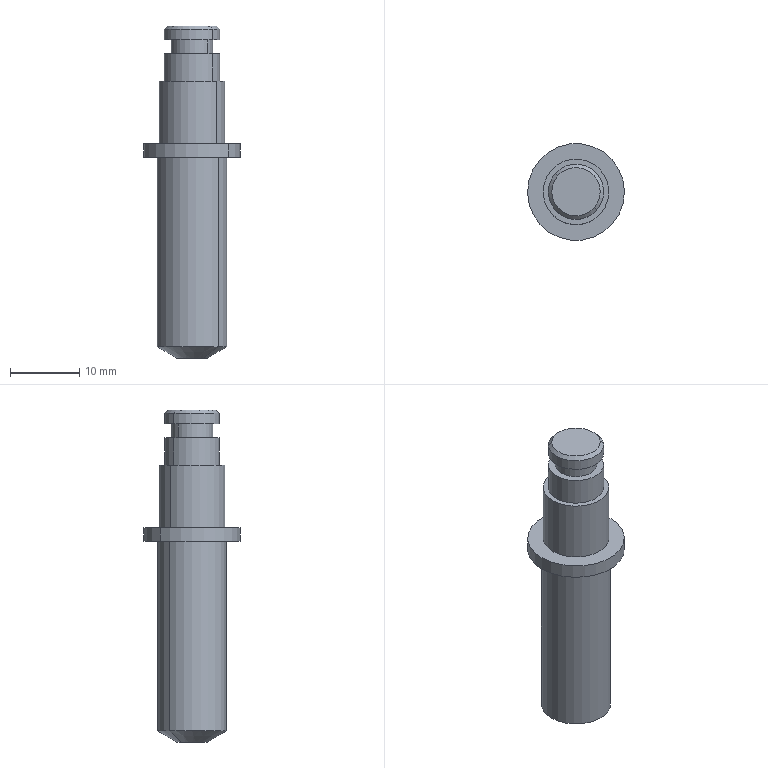Part | SolidWorks | features BaseBody 1 | 1 solid | 23 faces | box 14 x 14 x 48 mm | volume 3521 mm3 | cylinder 12 | plane 7 | cone 4 | commonest cylinder face diameters 8 x4 6 x2 9.5 x2 10 x2 14 x2
STEP:
#1=CARTESIAN_POINT('',(169.864,2.303,72.65));
#2=VERTEX_POINT('',#1);
#3=CARTESIAN_POINT('',(175.136,-2.303,72.65));
#4=VERTEX_POINT('',#3);
#5=CARTESIAN_POINT('',(172.5,0.,72.65));
#6=DIRECTION('',(0.,0.,1.));
#7=DIRECTION('',(0.7531,-0.6579,0.));
#8=AXIS2_PLACEMENT_3D('',#5,#6,#7);
#9=CIRCLE('',#8,3.5);
#10=EDGE_CURVE('',#2,#4,#9,.T.);
#11=ORIENTED_EDGE('',*,*,#10,.F.);
#12=CARTESIAN_POINT('',(169.488,2.632,72.15));
#13=VERTEX_POINT('',#12);
#14=CARTESIAN_POINT('',(169.488,2.632,72.15));
#15=DIRECTION('',(-0.5325,0.4652,-0.7071));
#16=VECTOR('',#15,1000.);
#17=LINE('',#14,#16);
#18=EDGE_CURVE('',#2,#13,#17,.T.);
#19=ORIENTED_EDGE('',*,*,#18,.T.);
#20=CARTESIAN_POINT('',(175.512,-2.632,72.15));
#21=VERTEX_POINT('',#20);
#22=CARTESIAN_POINT('',(172.5,0.,72.15));
#23=DIRECTION('',(0.,0.,-1.));
#24=DIRECTION('',(0.7531,-0.6579,0.));
#25=AXIS2_PLACEMENT_3D('',#22,#23,#24);
#26=CIRCLE('',#25,4.);
#27=EDGE_CURVE('',#21,#13,#26,.T.);
#28=ORIENTED_EDGE('',*,*,#27,.F.);
#29=CARTESIAN_POINT('',(175.512,-2.632,72.15));
#30=DIRECTION('',(0.5325,-0.4652,-0.7071));
#31=VECTOR('',#30,1000.);
#32=LINE('',#29,#31);
#33=EDGE_CURVE('',#4,#21,#32,.T.);
#34=ORIENTED_EDGE('',*,*,#33,.F.);
#35=EDGE_LOOP('',(#11,#19,#28,#34));
#36=FACE_OUTER_BOUND('',#35,.T.);
#37=CARTESIAN_POINT('',(172.5,0.,72.15));
#38=DIRECTION('',(0.,0.,-1.));
#39=DIRECTION('',(0.7531,-0.6579,0.));
#40=AXIS2_PLACEMENT_3D('',#37,#38,#39);
#41=CONICAL_SURFACE('',#40,4.,0.7854);
#42=ADVANCED_FACE('',(#36),#41,.T.);
#43=ORIENTED_EDGE('',*,*,#27,.T.);
#44=CARTESIAN_POINT('',(169.488,2.632,70.65));
#45=VERTEX_POINT('',#44);
#46=CARTESIAN_POINT('',(169.488,2.632,21.94));
#47=DIRECTION('',(0.,0.,-1.));
#48=VECTOR('',#47,1000.);
#49=LINE('',#46,#48);
#50=EDGE_CURVE('',#13,#45,#49,.T.);
#51=ORIENTED_EDGE('',*,*,#50,.T.);
#52=CARTESIAN_POINT('',(175.512,-2.632,70.65));
#53=VERTEX_POINT('',#52);
#54=CARTESIAN_POINT('',(172.5,0.,70.65));
#55=DIRECTION('',(0.,0.,-1.));
#56=DIRECTION('',(0.7531,-0.6579,0.));
#57=AXIS2_PLACEMENT_3D('',#54,#55,#56);
#58=CIRCLE('',#57,4.);
#59=EDGE_CURVE('',#53,#45,#58,.T.);
#60=ORIENTED_EDGE('',*,*,#59,.F.);
#61=CARTESIAN_POINT('',(175.512,-2.632,21.94));
#62=DIRECTION('',(0.,0.,-1.));
#63=VECTOR('',#62,1000.);
#64=LINE('',#61,#63);
#65=EDGE_CURVE('',#21,#53,#64,.T.);
#66=ORIENTED_EDGE('',*,*,#65,.F.);
#67=EDGE_LOOP('',(#43,#51,#60,#66));
#68=FACE_OUTER_BOUND('',#67,.T.);
#69=CARTESIAN_POINT('',(172.5,0.,21.94));
#70=DIRECTION('',(0.,0.,-1.));
#71=DIRECTION('',(0.7531,-0.6579,0.));
#72=AXIS2_PLACEMENT_3D('',#69,#70,#71);
#73=CYLINDRICAL_SURFACE('',#72,4.);
#74=ADVANCED_FACE('',(#68),#73,.T.);
#75=CARTESIAN_POINT('',(174.759,-1.974,70.65));
#76=VERTEX_POINT('',#75);
#77=CARTESIAN_POINT('',(170.241,1.974,70.65));
#78=VERTEX_POINT('',#77);
#79=CARTESIAN_POINT('',(172.5,0.,70.65));
#80=DIRECTION('',(0.,0.,-1.));
#81=DIRECTION('',(0.7531,-0.6579,0.));
#82=AXIS2_PLACEMENT_3D('',#79,#80,#81);
#83=CIRCLE('',#82,3.);
#84=EDGE_CURVE('',#76,#78,#83,.T.);
#85=ORIENTED_EDGE('',*,*,#84,.T.);
#86=CARTESIAN_POINT('',(170.241,1.974,68.65));
#87=VERTEX_POINT('',#86);
#88=CARTESIAN_POINT('',(170.241,1.974,21.94));
#89=DIRECTION('',(0.,0.,-1.));
#90=VECTOR('',#89,1000.);
#91=LINE('',#88,#90);
#92=EDGE_CURVE('',#78,#87,#91,.T.);
#93=ORIENTED_EDGE('',*,*,#92,.T.);
#94=CARTESIAN_POINT('',(174.759,-1.974,68.65));
#95=VERTEX_POINT('',#94);
#96=CARTESIAN_POINT('',(172.5,0.,68.65));
#97=DIRECTION('',(0.,0.,-1.));
#98=DIRECTION('',(0.7531,-0.6579,0.));
#99=AXIS2_PLACEMENT_3D('',#96,#97,#98);
#100=CIRCLE('',#99,3.);
#101=EDGE_CURVE('',#95,#87,#100,.T.);
#102=ORIENTED_EDGE('',*,*,#101,.F.);
#103=CARTESIAN_POINT('',(174.759,-1.974,21.94));
#104=DIRECTION('',(0.,0.,-1.));
#105=VECTOR('',#104,1000.);
#106=LINE('',#103,#105);
#107=EDGE_CURVE('',#76,#95,#106,.T.);
#108=ORIENTED_EDGE('',*,*,#107,.F.);
#109=EDGE_LOOP('',(#85,#93,#102,#108));
#110=FACE_OUTER_BOUND('',#109,.T.);
#111=CARTESIAN_POINT('',(172.5,0.,21.94));
#112=DIRECTION('',(0.,0.,-1.));
#113=DIRECTION('',(0.7531,-0.6579,0.));
#114=AXIS2_PLACEMENT_3D('',#111,#112,#113);
#115=CYLINDRICAL_SURFACE('',#114,3.);
#116=ADVANCED_FACE('',(#110),#115,.T.);
#117=CARTESIAN_POINT('',(175.512,-2.632,68.65));
#118=VERTEX_POINT('',#117);
#119=CARTESIAN_POINT('',(169.488,2.632,68.65));
#120=VERTEX_POINT('',#119);
#121=CARTESIAN_POINT('',(172.5,0.,68.65));
#122=DIRECTION('',(0.,0.,-1.));
#123=DIRECTION('',(0.7531,-0.6579,0.));
#124=AXIS2_PLACEMENT_3D('',#121,#122,#123);
#125=CIRCLE('',#124,4.);
#126=EDGE_CURVE('',#118,#120,#125,.T.);
#127=ORIENTED_EDGE('',*,*,#126,.T.);
#128=CARTESIAN_POINT('',(169.488,2.632,64.65));
#129=VERTEX_POINT('',#128);
#130=CARTESIAN_POINT('',(169.488,2.632,21.94));
#131=DIRECTION('',(0.,0.,-1.));
#132=VECTOR('',#131,1000.);
#133=LINE('',#130,#132);
#134=EDGE_CURVE('',#120,#129,#133,.T.);
#135=ORIENTED_EDGE('',*,*,#134,.T.);
#136=CARTESIAN_POINT('',(175.512,-2.632,64.65));
#137=VERTEX_POINT('',#136);
#138=CARTESIAN_POINT('',(172.5,0.,64.65));
#139=DIRECTION('',(0.,0.,-1.));
#140=DIRECTION('',(0.7531,-0.6579,0.));
#141=AXIS2_PLACEMENT_3D('',#138,#139,#140);
#142=CIRCLE('',#141,4.);
#143=EDGE_CURVE('',#137,#129,#142,.T.);
#144=ORIENTED_EDGE('',*,*,#143,.F.);
#145=CARTESIAN_POINT('',(175.512,-2.632,21.94));
#146=DIRECTION('',(0.,0.,-1.));
#147=VECTOR('',#146,1000.);
#148=LINE('',#145,#147);
#149=EDGE_CURVE('',#118,#137,#148,.T.);
#150=ORIENTED_EDGE('',*,*,#149,.F.);
#151=EDGE_LOOP('',(#127,#135,#144,#150));
#152=FACE_OUTER_BOUND('',#151,.T.);
#153=CARTESIAN_POINT('',(172.5,0.,21.94));
#154=DIRECTION('',(0.,0.,-1.));
#155=DIRECTION('',(0.7531,-0.6579,0.));
#156=AXIS2_PLACEMENT_3D('',#153,#154,#155);
#157=CYLINDRICAL_SURFACE('',#156,4.);
#158=ADVANCED_FACE('',(#152),#157,.T.);
#159=CARTESIAN_POINT('',(176.077,-3.125,64.65));
#160=VERTEX_POINT('',#159);
#161=CARTESIAN_POINT('',(168.923,3.125,64.65));
#162=VERTEX_POINT('',#161);
#163=CARTESIAN_POINT('',(172.5,0.,64.65));
#164=DIRECTION('',(0.,0.,-1.));
#165=DIRECTION('',(0.7531,-0.6579,0.));
#166=AXIS2_PLACEMENT_3D('',#163,#164,#165);
#167=CIRCLE('',#166,4.75);
#168=EDGE_CURVE('',#160,#162,#167,.T.);
#169=ORIENTED_EDGE('',*,*,#168,.T.);
#170=CARTESIAN_POINT('',(168.923,3.125,55.65));
#171=VERTEX_POINT('',#170);
#172=CARTESIAN_POINT('',(168.923,3.125,21.94));
#173=DIRECTION('',(0.,0.,-1.));
#174=VECTOR('',#173,1000.);
#175=LINE('',#172,#174);
#176=EDGE_CURVE('',#162,#171,#175,.T.);
#177=ORIENTED_EDGE('',*,*,#176,.T.);
#178=CARTESIAN_POINT('',(176.077,-3.125,55.65));
#179=VERTEX_POINT('',#178);
#180=CARTESIAN_POINT('',(172.5,0.,55.65));
#181=DIRECTION('',(0.,0.,-1.));
#182=DIRECTION('',(0.7531,-0.6579,0.));
#183=AXIS2_PLACEMENT_3D('',#180,#181,#182);
#184=CIRCLE('',#183,4.75);
#185=EDGE_CURVE('',#179,#171,#184,.T.);
#186=ORIENTED_EDGE('',*,*,#185,.F.);
#187=CARTESIAN_POINT('',(176.077,-3.125,21.94));
#188=DIRECTION('',(0.,0.,-1.));
#189=VECTOR('',#188,1000.);
#190=LINE('',#187,#189);
#191=EDGE_CURVE('',#160,#179,#190,.T.);
#192=ORIENTED_EDGE('',*,*,#191,.F.);
#193=EDGE_LOOP('',(#169,#177,#186,#192));
#194=FACE_OUTER_BOUND('',#193,.T.);
#195=CARTESIAN_POINT('',(172.5,0.,21.94));
#196=DIRECTION('',(0.,0.,-1.));
#197=DIRECTION('',(0.7531,-0.6579,0.));
#198=AXIS2_PLACEMENT_3D('',#195,#196,#197);
#199=CYLINDRICAL_SURFACE('',#198,4.75);
#200=ADVANCED_FACE('',(#194),#199,.T.);
#201=CARTESIAN_POINT('',(177.772,-4.605,55.65));
#202=VERTEX_POINT('',#201);
#203=CARTESIAN_POINT('',(167.228,4.605,55.65));
#204=VERTEX_POINT('',#203);
#205=CARTESIAN_POINT('',(172.5,0.,55.65));
#206=DIRECTION('',(0.,0.,-1.));
#207=DIRECTION('',(0.7531,-0.6579,0.));
#208=AXIS2_PLACEMENT_3D('',#205,#206,#207);
#209=CIRCLE('',#208,7.);
#210=EDGE_CURVE('',#202,#204,#209,.T.);
#211=ORIENTED_EDGE('',*,*,#210,.T.);
#212=CARTESIAN_POINT('',(167.228,4.605,53.65));
#213=VERTEX_POINT('',#212);
#214=CARTESIAN_POINT('',(167.228,4.605,21.94));
#215=DIRECTION('',(0.,0.,-1.));
#216=VECTOR('',#215,1000.);
#217=LINE('',#214,#216);
#218=EDGE_CURVE('',#204,#213,#217,.T.);
#219=ORIENTED_EDGE('',*,*,#218,.T.);
#220=CARTESIAN_POINT('',(177.772,-4.605,53.65));
#221=VERTEX_POINT('',#220);
#222=CARTESIAN_POINT('',(172.5,0.,53.65));
#223=DIRECTION('',(0.,0.,-1.));
#224=DIRECTION('',(0.7531,-0.6579,0.));
#225=AXIS2_PLACEMENT_3D('',#222,#223,#224);
#226=CIRCLE('',#225,7.);
#227=EDGE_CURVE('',#221,#213,#226,.T.);
#228=ORIENTED_EDGE('',*,*,#227,.F.);
#229=CARTESIAN_POINT('',(177.772,-4.605,21.94));
#230=DIRECTION('',(0.,0.,-1.));
#231=VECTOR('',#230,1000.);
#232=LINE('',#229,#231);
#233=EDGE_CURVE('',#202,#221,#232,.T.);
#234=ORIENTED_EDGE('',*,*,#233,.F.);
#235=EDGE_LOOP('',(#211,#219,#228,#234));
#236=FACE_OUTER_BOUND('',#235,.T.);
#237=CARTESIAN_POINT('',(172.5,0.,21.94));
#238=DIRECTION('',(0.,0.,-1.));
#239=DIRECTION('',(0.7531,-0.6579,0.));
#240=AXIS2_PLACEMENT_3D('',#237,#238,#239);
#241=CYLINDRICAL_SURFACE('',#240,7.);
#242=ADVANCED_FACE('',(#236),#241,.T.);
#243=CARTESIAN_POINT('',(176.266,-3.289,53.65));
#244=VERTEX_POINT('',#243);
#245=CARTESIAN_POINT('',(168.734,3.289,53.65));
#246=VERTEX_POINT('',#245);
#247=CARTESIAN_POINT('',(172.5,0.,53.65));
#248=DIRECTION('',(0.,0.,-1.));
#249=DIRECTION('',(0.7531,-0.6579,0.));
#250=AXIS2_PLACEMENT_3D('',#247,#248,#249);
#251=CIRCLE('',#250,5.);
#252=EDGE_CURVE('',#244,#246,#251,.T.);
#253=ORIENTED_EDGE('',*,*,#252,.T.);
#254=CARTESIAN_POINT('',(168.734,3.289,26.267));
#255=VERTEX_POINT('',#254);
#256=CARTESIAN_POINT('',(168.734,3.289,21.94));
#257=DIRECTION('',(0.,0.,-1.));
#258=VECTOR('',#257,1000.);
#259=LINE('',#256,#258);
#260=EDGE_CURVE('',#246,#255,#259,.T.);
#261=ORIENTED_EDGE('',*,*,#260,.T.);
#262=CARTESIAN_POINT('',(176.266,-3.289,26.267));
#263=VERTEX_POINT('',#262);
#264=CARTESIAN_POINT('',(172.5,0.,26.267));
#265=DIRECTION('',(0.,0.,-1.));
#266=DIRECTION('',(0.7531,-0.6579,0.));
#267=AXIS2_PLACEMENT_3D('',#264,#265,#266);
#268=CIRCLE('',#267,5.);
#269=EDGE_CURVE('',#263,#255,#268,.T.);
#270=ORIENTED_EDGE('',*,*,#269,.F.);
#271=CARTESIAN_POINT('',(176.266,-3.289,21.94));
#272=DIRECTION('',(0.,0.,-1.));
#273=VECTOR('',#272,1000.);
#274=LINE('',#271,#273);
#275=EDGE_CURVE('',#244,#263,#274,.T.);
#276=ORIENTED_EDGE('',*,*,#275,.F.);
#277=EDGE_LOOP('',(#253,#261,#270,#276));
#278=FACE_OUTER_BOUND('',#277,.T.);
#279=CARTESIAN_POINT('',(172.5,0.,21.94));
#280=DIRECTION('',(0.,0.,-1.));
#281=DIRECTION('',(0.7531,-0.6579,0.));
#282=AXIS2_PLACEMENT_3D('',#279,#280,#281);
#283=CYLINDRICAL_SURFACE('',#282,5.);
#284=ADVANCED_FACE('',(#278),#283,.T.);
#285=CARTESIAN_POINT('',(174.157,-1.447,24.65));
#286=VERTEX_POINT('',#285);
#287=CARTESIAN_POINT('',(170.843,1.447,24.65));
#288=VERTEX_POINT('',#287);
#289=CARTESIAN_POINT('',(172.5,0.,24.65));
#290=DIRECTION('',(0.,0.,-1.));
#291=DIRECTION('',(0.7531,-0.6579,0.));
#292=AXIS2_PLACEMENT_3D('',#289,#290,#291);
#293=CIRCLE('',#292,2.2);
#294=EDGE_CURVE('',#286,#288,#293,.T.);
#295=ORIENTED_EDGE('',*,*,#294,.F.);
#296=CARTESIAN_POINT('',(176.266,-3.289,26.267));
#297=DIRECTION('',(0.6522,-0.5697,0.5));
#298=VECTOR('',#297,1000.);
#299=LINE('',#296,#298);
#300=EDGE_CURVE('',#286,#263,#299,.T.);
#301=ORIENTED_EDGE('',*,*,#300,.T.);
#302=ORIENTED_EDGE('',*,*,#269,.T.);
#303=CARTESIAN_POINT('',(168.734,3.289,26.267));
#304=DIRECTION('',(-0.6522,0.5697,0.5));
#305=VECTOR('',#304,1000.);
#306=LINE('',#303,#305);
#307=EDGE_CURVE('',#288,#255,#306,.T.);
#308=ORIENTED_EDGE('',*,*,#307,.F.);
#309=EDGE_LOOP('',(#295,#301,#302,#308));
#310=FACE_OUTER_BOUND('',#309,.T.);
#311=CARTESIAN_POINT('',(172.5,0.,26.267));
#312=DIRECTION('',(0.,0.,1.));
#313=DIRECTION('',(-0.7531,0.6579,0.));
#314=AXIS2_PLACEMENT_3D('',#311,#312,#313);
#315=CONICAL_SURFACE('',#314,5.,1.047);
#316=ADVANCED_FACE('',(#310),#315,.T.);
#317=CARTESIAN_POINT('',(172.5,0.,24.65));
#318=DIRECTION('',(0.,0.,-1.));
#319=DIRECTION('',(0.7531,-0.6579,0.));
#320=AXIS2_PLACEMENT_3D('',#317,#318,#319);
#321=CIRCLE('',#320,2.2);
#322=EDGE_CURVE('',#288,#286,#321,.T.);
#323=ORIENTED_EDGE('',*,*,#322,.T.);
#324=ORIENTED_EDGE('',*,*,#294,.T.);
#325=EDGE_LOOP('',(#323,#324));
#326=FACE_OUTER_BOUND('',#325,.T.);
#327=CARTESIAN_POINT('',(172.5,0.,24.65));
#328=DIRECTION('',(0.,0.,1.));
#329=DIRECTION('',(-0.7531,0.6579,0.));
#330=AXIS2_PLACEMENT_3D('',#327,#328,#329);
#331=PLANE('',#330);
#332=ADVANCED_FACE('',(#326),#331,.F.);
#333=ORIENTED_EDGE('',*,*,#300,.F.);
#334=ORIENTED_EDGE('',*,*,#322,.F.);
#335=ORIENTED_EDGE('',*,*,#307,.T.);
#336=CARTESIAN_POINT('',(172.5,0.,26.267));
#337=DIRECTION('',(0.,0.,-1.));
#338=DIRECTION('',(0.7531,-0.6579,0.));
#339=AXIS2_PLACEMENT_3D('',#336,#337,#338);
#340=CIRCLE('',#339,5.);
#341=EDGE_CURVE('',#255,#263,#340,.T.);
#342=ORIENTED_EDGE('',*,*,#341,.T.);
#343=EDGE_LOOP('',(#333,#334,#335,#342));
#344=FACE_OUTER_BOUND('',#343,.T.);
#345=CARTESIAN_POINT('',(172.5,0.,26.267));
#346=DIRECTION('',(0.,0.,1.));
#347=DIRECTION('',(-0.7531,0.6579,0.));
#348=AXIS2_PLACEMENT_3D('',#345,#346,#347);
#349=CONICAL_SURFACE('',#348,5.,1.047);
#350=ADVANCED_FACE('',(#344),#349,.T.);
#351=ORIENTED_EDGE('',*,*,#260,.F.);
#352=CARTESIAN_POINT('',(172.5,0.,53.65));
#353=DIRECTION('',(0.,0.,-1.));
#354=DIRECTION('',(0.7531,-0.6579,0.));
#355=AXIS2_PLACEMENT_3D('',#352,#353,#354);
#356=CIRCLE('',#355,5.);
#357=EDGE_CURVE('',#246,#244,#356,.T.);
#358=ORIENTED_EDGE('',*,*,#357,.T.);
#359=ORIENTED_EDGE('',*,*,#275,.T.);
#360=ORIENTED_EDGE('',*,*,#341,.F.);
#361=EDGE_LOOP('',(#351,#358,#359,#360));
#362=FACE_OUTER_BOUND('',#361,.T.);
#363=CARTESIAN_POINT('',(172.5,0.,21.94));
#364=DIRECTION('',(0.,0.,-1.));
#365=DIRECTION('',(0.7531,-0.6579,0.));
#366=AXIS2_PLACEMENT_3D('',#363,#364,#365);
#367=CYLINDRICAL_SURFACE('',#366,5.);
#368=ADVANCED_FACE('',(#362),#367,.T.);
#369=ORIENTED_EDGE('',*,*,#252,.F.);
#370=ORIENTED_EDGE('',*,*,#357,.F.);
#371=EDGE_LOOP('',(#369,#370));
#372=FACE_BOUND('',#371,.T.);
#373=ORIENTED_EDGE('',*,*,#227,.T.);
#374=CARTESIAN_POINT('',(172.5,0.,53.65));
#375=DIRECTION('',(0.,0.,-1.));
#376=DIRECTION('',(0.7531,-0.6579,0.));
#377=AXIS2_PLACEMENT_3D('',#374,#375,#376);
#378=CIRCLE('',#377,7.);
#379=EDGE_CURVE('',#213,#221,#378,.T.);
#380=ORIENTED_EDGE('',*,*,#379,.T.);
#381=EDGE_LOOP('',(#373,#380));
#382=FACE_OUTER_BOUND('',#381,.T.);
#383=CARTESIAN_POINT('',(169.211,-3.766,53.65));
#384=DIRECTION('',(0.,0.,1.));
#385=DIRECTION('',(-0.7531,0.6579,0.));
#386=AXIS2_PLACEMENT_3D('',#383,#384,#385);
#387=PLANE('',#386);
#388=ADVANCED_FACE('',(#372,#382),#387,.F.);
#389=ORIENTED_EDGE('',*,*,#218,.F.);
#390=CARTESIAN_POINT('',(172.5,0.,55.65));
#391=DIRECTION('',(0.,0.,-1.));
#392=DIRECTION('',(0.7531,-0.6579,0.));
#393=AXIS2_PLACEMENT_3D('',#390,#391,#392);
#394=CIRCLE('',#393,7.);
#395=EDGE_CURVE('',#204,#202,#394,.T.);
#396=ORIENTED_EDGE('',*,*,#395,.T.);
#397=ORIENTED_EDGE('',*,*,#233,.T.);
#398=ORIENTED_EDGE('',*,*,#379,.F.);
#399=EDGE_LOOP('',(#389,#396,#397,#398));
#400=FACE_OUTER_BOUND('',#399,.T.);
#401=CARTESIAN_POINT('',(172.5,0.,21.94));
#402=DIRECTION('',(0.,0.,-1.));
#403=DIRECTION('',(0.7531,-0.6579,0.));
#404=AXIS2_PLACEMENT_3D('',#401,#402,#403);
#405=CYLINDRICAL_SURFACE('',#404,7.);
#406=ADVANCED_FACE('',(#400),#405,.T.);
#407=ORIENTED_EDGE('',*,*,#210,.F.);
#408=ORIENTED_EDGE('',*,*,#395,.F.);
#409=EDGE_LOOP('',(#407,#408));
#410=FACE_OUTER_BOUND('',#409,.T.);
#411=ORIENTED_EDGE('',*,*,#185,.T.);
#412=CARTESIAN_POINT('',(172.5,0.,55.65));
#413=DIRECTION('',(0.,0.,-1.));
#414=DIRECTION('',(0.7531,-0.6579,0.));
#415=AXIS2_PLACEMENT_3D('',#412,#413,#414);
#416=CIRCLE('',#415,4.75);
#417=EDGE_CURVE('',#171,#179,#416,.T.);
#418=ORIENTED_EDGE('',*,*,#417,.T.);
#419=EDGE_LOOP('',(#411,#418));
#420=FACE_BOUND('',#419,.T.);
#421=CARTESIAN_POINT('',(167.895,-5.272,55.65));
#422=DIRECTION('',(0.,0.,-1.));
#423=DIRECTION('',(0.7531,-0.6579,0.));
#424=AXIS2_PLACEMENT_3D('',#421,#422,#423);
#425=PLANE('',#424);
#426=ADVANCED_FACE('',(#410,#420),#425,.F.);
#427=ORIENTED_EDGE('',*,*,#176,.F.);
#428=CARTESIAN_POINT('',(172.5,0.,64.65));
#429=DIRECTION('',(0.,0.,-1.));
#430=DIRECTION('',(0.7531,-0.6579,0.));
#431=AXIS2_PLACEMENT_3D('',#428,#429,#430);
#432=CIRCLE('',#431,4.75);
#433=EDGE_CURVE('',#162,#160,#432,.T.);
#434=ORIENTED_EDGE('',*,*,#433,.T.);
#435=ORIENTED_EDGE('',*,*,#191,.T.);
#436=ORIENTED_EDGE('',*,*,#417,.F.);
#437=EDGE_LOOP('',(#427,#434,#435,#436));
#438=FACE_OUTER_BOUND('',#437,.T.);
#439=CARTESIAN_POINT('',(172.5,0.,21.94));
#440=DIRECTION('',(0.,0.,-1.));
#441=DIRECTION('',(0.7531,-0.6579,0.));
#442=AXIS2_PLACEMENT_3D('',#439,#440,#441);
#443=CYLINDRICAL_SURFACE('',#442,4.75);
#444=ADVANCED_FACE('',(#438),#443,.T.);
#445=ORIENTED_EDGE('',*,*,#168,.F.);
#446=ORIENTED_EDGE('',*,*,#433,.F.);
#447=EDGE_LOOP('',(#445,#446));
#448=FACE_OUTER_BOUND('',#447,.T.);
#449=ORIENTED_EDGE('',*,*,#143,.T.);
#450=CARTESIAN_POINT('',(172.5,0.,64.65));
#451=DIRECTION('',(0.,0.,-1.));
#452=DIRECTION('',(0.7531,-0.6579,0.));
#453=AXIS2_PLACEMENT_3D('',#450,#451,#452);
#454=CIRCLE('',#453,4.);
#455=EDGE_CURVE('',#129,#137,#454,.T.);
#456=ORIENTED_EDGE('',*,*,#455,.T.);
#457=EDGE_LOOP('',(#449,#456));
#458=FACE_BOUND('',#457,.T.);
#459=CARTESIAN_POINT('',(169.375,-3.577,64.65));
#460=DIRECTION('',(0.,0.,-1.));
#461=DIRECTION('',(0.7531,-0.6579,0.));
#462=AXIS2_PLACEMENT_3D('',#459,#460,#461);
#463=PLANE('',#462);
#464=ADVANCED_FACE('',(#448,#458),#463,.F.);
#465=ORIENTED_EDGE('',*,*,#134,.F.);
#466=CARTESIAN_POINT('',(172.5,0.,68.65));
#467=DIRECTION('',(0.,0.,-1.));
#468=DIRECTION('',(0.7531,-0.6579,0.));
#469=AXIS2_PLACEMENT_3D('',#466,#467,#468);
#470=CIRCLE('',#469,4.);
#471=EDGE_CURVE('',#120,#118,#470,.T.);
#472=ORIENTED_EDGE('',*,*,#471,.T.);
#473=ORIENTED_EDGE('',*,*,#149,.T.);
#474=ORIENTED_EDGE('',*,*,#455,.F.);
#475=EDGE_LOOP('',(#465,#472,#473,#474));
#476=FACE_OUTER_BOUND('',#475,.T.);
#477=CARTESIAN_POINT('',(172.5,0.,21.94));
#478=DIRECTION('',(0.,0.,-1.));
#479=DIRECTION('',(0.7531,-0.6579,0.));
#480=AXIS2_PLACEMENT_3D('',#477,#478,#479);
#481=CYLINDRICAL_SURFACE('',#480,4.);
#482=ADVANCED_FACE('',(#476),#481,.T.);
#483=ORIENTED_EDGE('',*,*,#126,.F.);
#484=ORIENTED_EDGE('',*,*,#471,.F.);
#485=EDGE_LOOP('',(#483,#484));
#486=FACE_OUTER_BOUND('',#485,.T.);
#487=ORIENTED_EDGE('',*,*,#101,.T.);
#488=CARTESIAN_POINT('',(172.5,0.,68.65));
#489=DIRECTION('',(0.,0.,-1.));
#490=DIRECTION('',(0.7531,-0.6579,0.));
#491=AXIS2_PLACEMENT_3D('',#488,#489,#490);
#492=CIRCLE('',#491,3.);
#493=EDGE_CURVE('',#87,#95,#492,.T.);
#494=ORIENTED_EDGE('',*,*,#493,.T.);
#495=EDGE_LOOP('',(#487,#494));
#496=FACE_BOUND('',#495,.T.);
#497=CARTESIAN_POINT('',(169.868,-3.012,68.65));
#498=DIRECTION('',(0.,0.,-1.));
#499=DIRECTION('',(0.7531,-0.6579,0.));
#500=AXIS2_PLACEMENT_3D('',#497,#498,#499);
#501=PLANE('',#500);
#502=ADVANCED_FACE('',(#486,#496),#501,.F.);
#503=ORIENTED_EDGE('',*,*,#92,.F.);
#504=CARTESIAN_POINT('',(172.5,0.,70.65));
#505=DIRECTION('',(0.,0.,-1.));
#506=DIRECTION('',(0.7531,-0.6579,0.));
#507=AXIS2_PLACEMENT_3D('',#504,#505,#506);
#508=CIRCLE('',#507,3.);
#509=EDGE_CURVE('',#78,#76,#508,.T.);
#510=ORIENTED_EDGE('',*,*,#509,.T.);
#511=ORIENTED_EDGE('',*,*,#107,.T.);
#512=ORIENTED_EDGE('',*,*,#493,.F.);
#513=EDGE_LOOP('',(#503,#510,#511,#512));
#514=FACE_OUTER_BOUND('',#513,.T.);
#515=CARTESIAN_POINT('',(172.5,0.,21.94));
#516=DIRECTION('',(0.,0.,-1.));
#517=DIRECTION('',(0.7531,-0.6579,0.));
#518=AXIS2_PLACEMENT_3D('',#515,#516,#517);
#519=CYLINDRICAL_SURFACE('',#518,3.);
#520=ADVANCED_FACE('',(#514),#519,.T.);
#521=ORIENTED_EDGE('',*,*,#84,.F.);
#522=ORIENTED_EDGE('',*,*,#509,.F.);
#523=EDGE_LOOP('',(#521,#522));
#524=FACE_BOUND('',#523,.T.);
#525=ORIENTED_EDGE('',*,*,#59,.T.);
#526=CARTESIAN_POINT('',(172.5,0.,70.65));
#527=DIRECTION('',(0.,0.,-1.));
#528=DIRECTION('',(0.7531,-0.6579,0.));
#529=AXIS2_PLACEMENT_3D('',#526,#527,#528);
#530=CIRCLE('',#529,4.);
#531=EDGE_CURVE('',#45,#53,#530,.T.);
#532=ORIENTED_EDGE('',*,*,#531,.T.);
#533=EDGE_LOOP('',(#525,#532));
#534=FACE_OUTER_BOUND('',#533,.T.);
#535=CARTESIAN_POINT('',(170.526,-2.259,70.65));
#536=DIRECTION('',(0.,0.,1.));
#537=DIRECTION('',(-0.7531,0.6579,0.));
#538=AXIS2_PLACEMENT_3D('',#535,#536,#537);
#539=PLANE('',#538);
#540=ADVANCED_FACE('',(#524,#534),#539,.F.);
#541=ORIENTED_EDGE('',*,*,#50,.F.);
#542=CARTESIAN_POINT('',(172.5,0.,72.15));
#543=DIRECTION('',(0.,0.,-1.));
#544=DIRECTION('',(0.7531,-0.6579,0.));
#545=AXIS2_PLACEMENT_3D('',#542,#543,#544);
#546=CIRCLE('',#545,4.);
#547=EDGE_CURVE('',#13,#21,#546,.T.);
#548=ORIENTED_EDGE('',*,*,#547,.T.);
#549=ORIENTED_EDGE('',*,*,#65,.T.);
#550=ORIENTED_EDGE('',*,*,#531,.F.);
#551=EDGE_LOOP('',(#541,#548,#549,#550));
#552=FACE_OUTER_BOUND('',#551,.T.);
#553=CARTESIAN_POINT('',(172.5,0.,21.94));
#554=DIRECTION('',(0.,0.,-1.));
#555=DIRECTION('',(0.7531,-0.6579,0.));
#556=AXIS2_PLACEMENT_3D('',#553,#554,#555);
#557=CYLINDRICAL_SURFACE('',#556,4.);
#558=ADVANCED_FACE('',(#552),#557,.T.);
#559=CARTESIAN_POINT('',(172.5,0.,72.65));
#560=DIRECTION('',(0.,0.,1.));
#561=DIRECTION('',(0.7531,-0.6579,0.));
#562=AXIS2_PLACEMENT_3D('',#559,#560,#561);
#563=CIRCLE('',#562,3.5);
#564=EDGE_CURVE('',#4,#2,#563,.T.);
#565=ORIENTED_EDGE('',*,*,#564,.T.);
#566=ORIENTED_EDGE('',*,*,#10,.T.);
#567=EDGE_LOOP('',(#565,#566));
#568=FACE_OUTER_BOUND('',#567,.T.);
#569=CARTESIAN_POINT('',(169.868,-3.012,72.65));
#570=DIRECTION('',(0.,0.,-1.));
#571=DIRECTION('',(0.7531,-0.6579,0.));
#572=AXIS2_PLACEMENT_3D('',#569,#570,#571);
#573=PLANE('',#572);
#574=ADVANCED_FACE('',(#568),#573,.F.);
#575=ORIENTED_EDGE('',*,*,#18,.F.);
#576=ORIENTED_EDGE('',*,*,#564,.F.);
#577=ORIENTED_EDGE('',*,*,#33,.T.);
#578=ORIENTED_EDGE('',*,*,#547,.F.);
#579=EDGE_LOOP('',(#575,#576,#577,#578));
#580=FACE_OUTER_BOUND('',#579,.T.);
#581=CARTESIAN_POINT('',(172.5,0.,72.15));
#582=DIRECTION('',(0.,0.,-1.));
#583=DIRECTION('',(0.7531,-0.6579,0.));
#584=AXIS2_PLACEMENT_3D('',#581,#582,#583);
#585=CONICAL_SURFACE('',#584,4.,0.7854);
#586=ADVANCED_FACE('',(#580),#585,.T.);
#587=CLOSED_SHELL('',(#42,#74,#116,#158,#200,#242,#284,#316,#332,#350,#368,#388,#406,#426,#444,#464,#482,#502,#520,#540,#558,#574,#586));
#588=MANIFOLD_SOLID_BREP('',#587);
#589=CARTESIAN_POINT('',(0.,0.,0.));
#590=DIRECTION('',(0.,0.,1.));
#591=DIRECTION('',(1.,0.,0.));
#592=AXIS2_PLACEMENT_3D('',#589,#590,#591);
#593=(LENGTH_UNIT()NAMED_UNIT(*)SI_UNIT(.MILLI.,.METRE.));
#594=UNCERTAINTY_MEASURE_WITH_UNIT(LENGTH_MEASURE(0.00001),#593,'','');
#595=(NAMED_UNIT(*)PLANE_ANGLE_UNIT()SI_UNIT($,.RADIAN.));
#596=(NAMED_UNIT(*)SI_UNIT($,.STERADIAN.)SOLID_ANGLE_UNIT());
#597=(GEOMETRIC_REPRESENTATION_CONTEXT(3)GLOBAL_UNCERTAINTY_ASSIGNED_CONTEXT((#594))GLOBAL_UNIT_ASSIGNED_CONTEXT((#593,#595,#596))REPRESENTATION_CONTEXT('',''));
#598=ADVANCED_BREP_SHAPE_REPRESENTATION('',(#588,#592),#597);